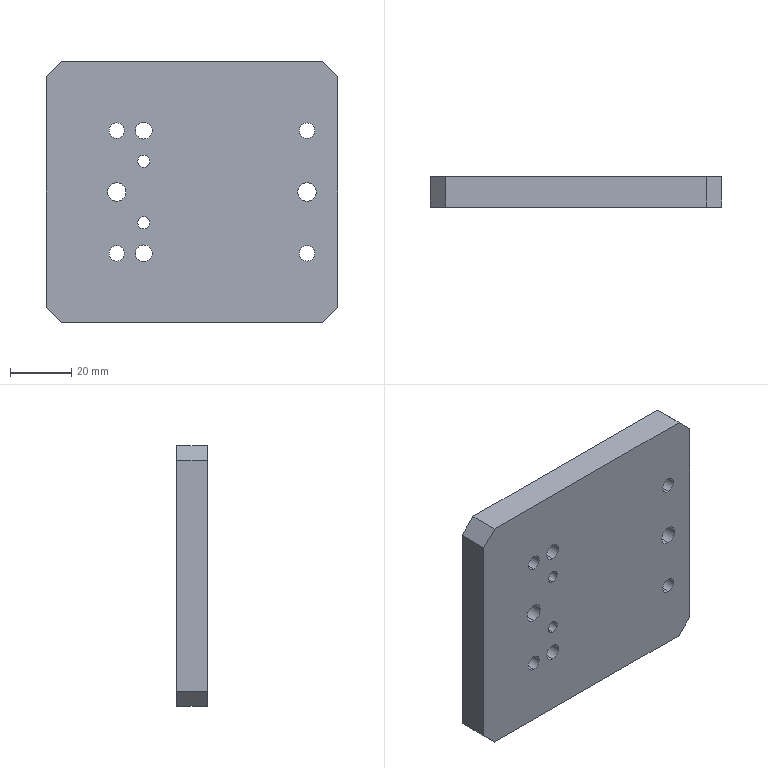Part | STEP file | PN_0022 | 1 solid | 36 faces | box 95 x 10 x 85 mm | volume 77581 mm3 | cylinder 24 | plane 12 | commonest cylinder face diameters 5 x8 4 x4 5.5 x4 6 x4 10 x4